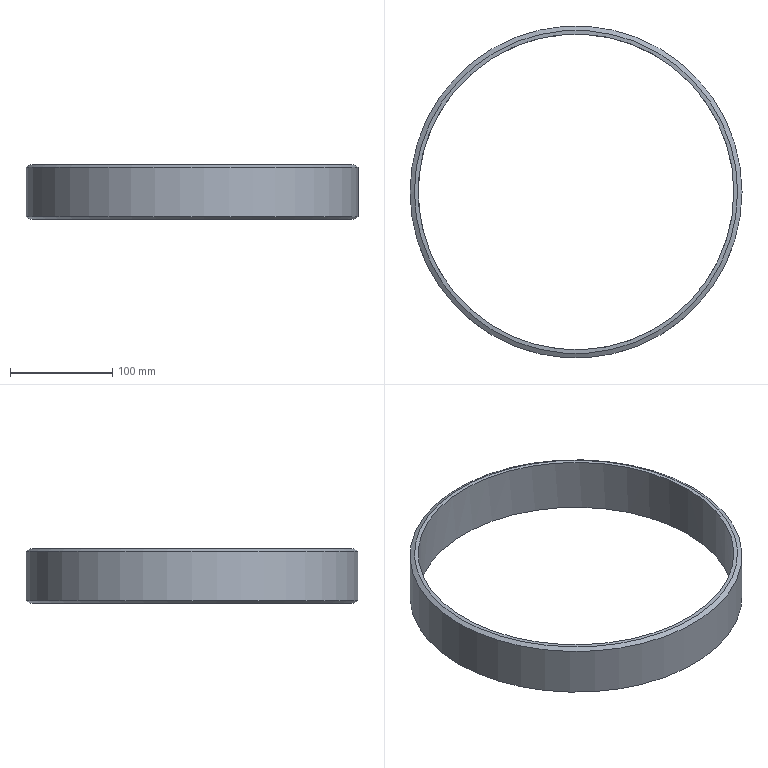Part | NX | features CHAMFER 1, CYLINDER 1, DATUM_CSYS 1, SHELL 1 | 1 solid | 6 faces | box 325 x 325 x 53.774 mm | volume 417463 mm3 | plane 2 | cylinder 2 | cone 2 | commonest cylinder face diameters 309 x1 325 x1
STEP:
#1=CARTESIAN_POINT('',(158.17,0.,53.773));
#2=VERTEX_POINT('',#1);
#3=CARTESIAN_POINT('',(0.,0.,53.773));
#4=DIRECTION('',(0.,0.,1.));
#5=DIRECTION('',(1.,0.,0.));
#6=AXIS2_PLACEMENT_3D('',#3,#4,#5);
#7=CIRCLE('',#6,158.17);
#8=EDGE_CURVE('',#2,#2,#7,.T.);
#9=ORIENTED_EDGE('',*,*,#8,.T.);
#10=EDGE_LOOP('',(#9));
#11=FACE_BOUND('',#10,.T.);
#12=CARTESIAN_POINT('',(154.5,0.,53.773));
#13=VERTEX_POINT('',#12);
#14=CARTESIAN_POINT('',(0.,0.,53.773));
#15=DIRECTION('',(0.,0.,1.));
#16=DIRECTION('',(1.,0.,0.));
#17=AXIS2_PLACEMENT_3D('',#14,#15,#16);
#18=CIRCLE('',#17,154.5);
#19=EDGE_CURVE('',#13,#13,#18,.F.);
#20=ORIENTED_EDGE('',*,*,#19,.T.);
#21=EDGE_LOOP('',(#20));
#22=FACE_BOUND('',#21,.T.);
#23=CARTESIAN_POINT('',(0.,0.,53.773));
#24=DIRECTION('',(0.,0.,1.));
#25=DIRECTION('',(1.,0.,0.));
#26=AXIS2_PLACEMENT_3D('',#23,#24,#25);
#27=PLANE('',#26);
#28=ADVANCED_FACE('',(#11,#22),#27,.T.);
#29=CARTESIAN_POINT('',(-158.17,0.,0.));
#30=VERTEX_POINT('',#29);
#31=CARTESIAN_POINT('',(0.,0.,0.));
#32=DIRECTION('',(0.,0.,-1.));
#33=DIRECTION('',(-1.,0.,0.));
#34=AXIS2_PLACEMENT_3D('',#31,#32,#33);
#35=CIRCLE('',#34,158.17);
#36=EDGE_CURVE('',#30,#30,#35,.T.);
#37=ORIENTED_EDGE('',*,*,#36,.T.);
#38=EDGE_LOOP('',(#37));
#39=FACE_BOUND('',#38,.T.);
#40=CARTESIAN_POINT('',(-154.5,0.,0.));
#41=VERTEX_POINT('',#40);
#42=CARTESIAN_POINT('',(0.,0.,0.));
#43=DIRECTION('',(0.,0.,-1.));
#44=DIRECTION('',(-1.,0.,0.));
#45=AXIS2_PLACEMENT_3D('',#42,#43,#44);
#46=CIRCLE('',#45,154.5);
#47=EDGE_CURVE('',#41,#41,#46,.F.);
#48=ORIENTED_EDGE('',*,*,#47,.T.);
#49=EDGE_LOOP('',(#48));
#50=FACE_BOUND('',#49,.T.);
#51=CARTESIAN_POINT('',(0.,0.,0.));
#52=DIRECTION('',(0.,0.,-1.));
#53=DIRECTION('',(-1.,0.,0.));
#54=AXIS2_PLACEMENT_3D('',#51,#52,#53);
#55=PLANE('',#54);
#56=ADVANCED_FACE('',(#39,#50),#55,.T.);
#57=CARTESIAN_POINT('',(-162.5,0.,2.5));
#58=VERTEX_POINT('',#57);
#59=CARTESIAN_POINT('',(0.,0.,2.5));
#60=DIRECTION('',(0.,0.,-1.));
#61=DIRECTION('',(-1.,0.,0.));
#62=AXIS2_PLACEMENT_3D('',#59,#60,#61);
#63=CIRCLE('',#62,162.5);
#64=EDGE_CURVE('',#58,#58,#63,.F.);
#65=ORIENTED_EDGE('',*,*,#64,.T.);
#66=EDGE_LOOP('',(#65));
#67=FACE_BOUND('',#66,.T.);
#68=CARTESIAN_POINT('',(162.5,0.,51.273));
#69=VERTEX_POINT('',#68);
#70=CARTESIAN_POINT('',(0.,0.,51.273));
#71=DIRECTION('',(0.,0.,1.));
#72=DIRECTION('',(1.,0.,0.));
#73=AXIS2_PLACEMENT_3D('',#70,#71,#72);
#74=CIRCLE('',#73,162.5);
#75=EDGE_CURVE('',#69,#69,#74,.F.);
#76=ORIENTED_EDGE('',*,*,#75,.T.);
#77=EDGE_LOOP('',(#76));
#78=FACE_BOUND('',#77,.T.);
#79=CARTESIAN_POINT('',(0.,0.,0.));
#80=DIRECTION('',(0.,0.,1.));
#81=DIRECTION('',(1.,0.,0.));
#82=AXIS2_PLACEMENT_3D('',#79,#80,#81);
#83=CYLINDRICAL_SURFACE('',#82,162.5);
#84=ADVANCED_FACE('',(#67,#78),#83,.T.);
#85=ORIENTED_EDGE('',*,*,#19,.F.);
#86=EDGE_LOOP('',(#85));
#87=FACE_BOUND('',#86,.T.);
#88=ORIENTED_EDGE('',*,*,#47,.F.);
#89=EDGE_LOOP('',(#88));
#90=FACE_BOUND('',#89,.T.);
#91=CARTESIAN_POINT('',(0.,0.,0.));
#92=DIRECTION('',(0.,0.,1.));
#93=DIRECTION('',(1.,0.,0.));
#94=AXIS2_PLACEMENT_3D('',#91,#92,#93);
#95=CYLINDRICAL_SURFACE('',#94,154.5);
#96=ADVANCED_FACE('',(#87,#90),#95,.F.);
#97=ORIENTED_EDGE('',*,*,#36,.F.);
#98=EDGE_LOOP('',(#97));
#99=FACE_BOUND('',#98,.T.);
#100=ORIENTED_EDGE('',*,*,#64,.F.);
#101=EDGE_LOOP('',(#100));
#102=FACE_BOUND('',#101,.T.);
#103=CARTESIAN_POINT('',(0.,0.,2.5));
#104=DIRECTION('',(0.,0.,1.));
#105=DIRECTION('',(1.,0.,0.));
#106=AXIS2_PLACEMENT_3D('',#103,#104,#105);
#107=CONICAL_SURFACE('',#106,162.5,1.047);
#108=ADVANCED_FACE('',(#99,#102),#107,.T.);
#109=ORIENTED_EDGE('',*,*,#8,.F.);
#110=EDGE_LOOP('',(#109));
#111=FACE_BOUND('',#110,.T.);
#112=ORIENTED_EDGE('',*,*,#75,.F.);
#113=EDGE_LOOP('',(#112));
#114=FACE_BOUND('',#113,.T.);
#115=CARTESIAN_POINT('',(0.,0.,51.273));
#116=DIRECTION('',(0.,0.,-1.));
#117=DIRECTION('',(-1.,0.,0.));
#118=AXIS2_PLACEMENT_3D('',#115,#116,#117);
#119=CONICAL_SURFACE('',#118,162.5,1.047);
#120=ADVANCED_FACE('',(#111,#114),#119,.T.);
#121=CLOSED_SHELL('',(#28,#56,#84,#96,#108,#120));
#122=MANIFOLD_SOLID_BREP('',#121);
#123=(LENGTH_UNIT()NAMED_UNIT(*)SI_UNIT(.MILLI.,.METRE.));
#124=UNCERTAINTY_MEASURE_WITH_UNIT(LENGTH_MEASURE(0.00001),#123,'','');
#125=(NAMED_UNIT(*)PLANE_ANGLE_UNIT()SI_UNIT($,.RADIAN.));
#126=(NAMED_UNIT(*)SI_UNIT($,.STERADIAN.)SOLID_ANGLE_UNIT());
#127=(GEOMETRIC_REPRESENTATION_CONTEXT(3)GLOBAL_UNCERTAINTY_ASSIGNED_CONTEXT((#124))GLOBAL_UNIT_ASSIGNED_CONTEXT((#123,#125,#126))REPRESENTATION_CONTEXT('',''));
#128=ADVANCED_BREP_SHAPE_REPRESENTATION('',(#122),#127);